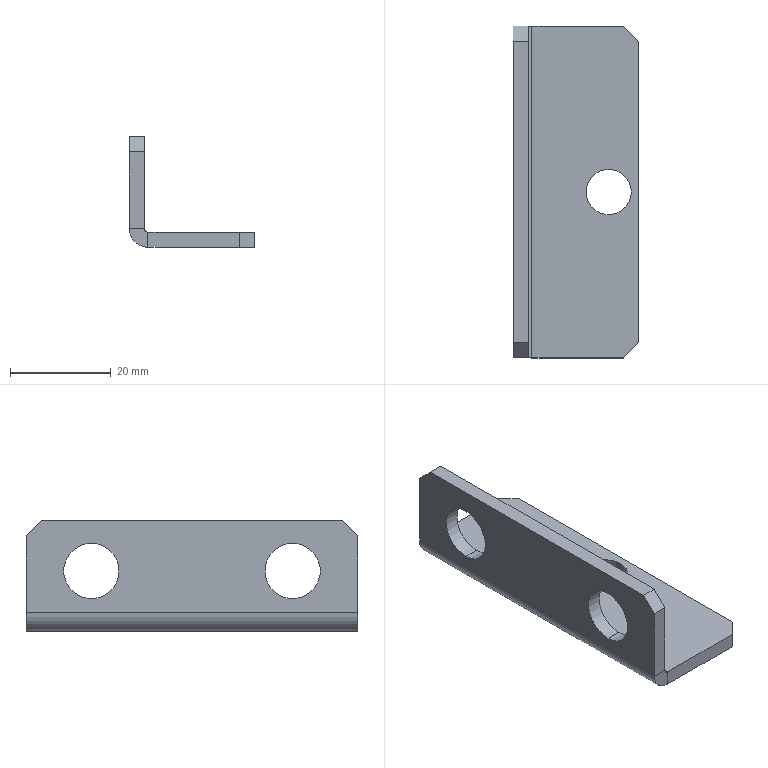Part | SolidWorks | features HoleWzd 2, 3DProfileFeature 1, BreakCorner 1, EdgeFlange 1, FlatPattern 1, SMBaseFlange 1, SheetMetal 1 | 1 solid | 24 faces | box 25 x 66 x 22 mm | volume 7707 mm3 | plane 16 | cylinder 8 | commonest cylinder face diameters 11 x4 9 x2 1.473 x1 7.473 x1
STEP:
#1=CARTESIAN_POINT('',(11.,0.,-3.));
#2=VERTEX_POINT('',#1);
#3=CARTESIAN_POINT('',(2.,0.,-3.));
#4=VERTEX_POINT('',#3);
#5=CARTESIAN_POINT('',(6.5,0.,-3.));
#6=DIRECTION('',(0.,0.,-1.));
#7=DIRECTION('',(-1.,0.,0.));
#8=AXIS2_PLACEMENT_3D('',#5,#6,#7);
#9=CIRCLE('',#8,4.5);
#10=EDGE_CURVE('',#2,#4,#9,.T.);
#11=ORIENTED_EDGE('',*,*,#10,.T.);
#12=CARTESIAN_POINT('',(2.,0.,0.));
#13=VERTEX_POINT('',#12);
#14=CARTESIAN_POINT('',(2.,0.,0.));
#15=DIRECTION('',(0.,0.,1.));
#16=VECTOR('',#15,1000.);
#17=LINE('',#14,#16);
#18=EDGE_CURVE('',#4,#13,#17,.T.);
#19=ORIENTED_EDGE('',*,*,#18,.T.);
#20=CARTESIAN_POINT('',(11.,0.,0.));
#21=VERTEX_POINT('',#20);
#22=CARTESIAN_POINT('',(6.5,0.,0.));
#23=DIRECTION('',(0.,0.,1.));
#24=DIRECTION('',(1.,0.,0.));
#25=AXIS2_PLACEMENT_3D('',#22,#23,#24);
#26=CIRCLE('',#25,4.5);
#27=EDGE_CURVE('',#13,#21,#26,.T.);
#28=ORIENTED_EDGE('',*,*,#27,.T.);
#29=CARTESIAN_POINT('',(11.,0.,0.));
#30=DIRECTION('',(0.,0.,1.));
#31=VECTOR('',#30,1000.);
#32=LINE('',#29,#31);
#33=EDGE_CURVE('',#2,#21,#32,.T.);
#34=ORIENTED_EDGE('',*,*,#33,.F.);
#35=EDGE_LOOP('',(#11,#19,#28,#34));
#36=FACE_OUTER_BOUND('',#35,.T.);
#37=CARTESIAN_POINT('',(6.5,0.,0.));
#38=DIRECTION('',(0.,0.,1.));
#39=DIRECTION('',(1.,0.,0.));
#40=AXIS2_PLACEMENT_3D('',#37,#38,#39);
#41=CYLINDRICAL_SURFACE('',#40,4.5);
#42=ADVANCED_FACE('',(#36),#41,.F.);
#43=CARTESIAN_POINT('',(-12.5,20.,14.5));
#44=VERTEX_POINT('',#43);
#45=CARTESIAN_POINT('',(-12.5,20.,3.5));
#46=VERTEX_POINT('',#45);
#47=CARTESIAN_POINT('',(-12.5,20.,9.));
#48=DIRECTION('',(1.,0.,0.));
#49=DIRECTION('',(0.,0.,-1.));
#50=AXIS2_PLACEMENT_3D('',#47,#48,#49);
#51=CIRCLE('',#50,5.5);
#52=EDGE_CURVE('',#44,#46,#51,.T.);
#53=ORIENTED_EDGE('',*,*,#52,.F.);
#54=CARTESIAN_POINT('',(-9.5,20.,14.5));
#55=VERTEX_POINT('',#54);
#56=CARTESIAN_POINT('',(-9.5,20.,14.5));
#57=DIRECTION('',(1.,0.,0.));
#58=VECTOR('',#57,1000.);
#59=LINE('',#56,#58);
#60=EDGE_CURVE('',#44,#55,#59,.T.);
#61=ORIENTED_EDGE('',*,*,#60,.T.);
#62=CARTESIAN_POINT('',(-9.5,20.,3.5));
#63=VERTEX_POINT('',#62);
#64=CARTESIAN_POINT('',(-9.5,20.,9.));
#65=DIRECTION('',(1.,0.,0.));
#66=DIRECTION('',(0.,0.,-1.));
#67=AXIS2_PLACEMENT_3D('',#64,#65,#66);
#68=CIRCLE('',#67,5.5);
#69=EDGE_CURVE('',#55,#63,#68,.T.);
#70=ORIENTED_EDGE('',*,*,#69,.T.);
#71=CARTESIAN_POINT('',(-9.5,20.,3.5));
#72=DIRECTION('',(1.,0.,0.));
#73=VECTOR('',#72,1000.);
#74=LINE('',#71,#73);
#75=EDGE_CURVE('',#46,#63,#74,.T.);
#76=ORIENTED_EDGE('',*,*,#75,.F.);
#77=EDGE_LOOP('',(#53,#61,#70,#76));
#78=FACE_OUTER_BOUND('',#77,.T.);
#79=CARTESIAN_POINT('',(-9.5,20.,9.));
#80=DIRECTION('',(1.,0.,0.));
#81=DIRECTION('',(0.,0.,-1.));
#82=AXIS2_PLACEMENT_3D('',#79,#80,#81);
#83=CYLINDRICAL_SURFACE('',#82,5.5);
#84=ADVANCED_FACE('',(#78),#83,.F.);
#85=CARTESIAN_POINT('',(-12.5,-20.,14.5));
#86=VERTEX_POINT('',#85);
#87=CARTESIAN_POINT('',(-12.5,-20.,3.5));
#88=VERTEX_POINT('',#87);
#89=CARTESIAN_POINT('',(-12.5,-20.,9.));
#90=DIRECTION('',(1.,0.,0.));
#91=DIRECTION('',(0.,0.,-1.));
#92=AXIS2_PLACEMENT_3D('',#89,#90,#91);
#93=CIRCLE('',#92,5.5);
#94=EDGE_CURVE('',#86,#88,#93,.T.);
#95=ORIENTED_EDGE('',*,*,#94,.F.);
#96=CARTESIAN_POINT('',(-9.5,-20.,14.5));
#97=VERTEX_POINT('',#96);
#98=CARTESIAN_POINT('',(-9.5,-20.,14.5));
#99=DIRECTION('',(1.,0.,0.));
#100=VECTOR('',#99,1000.);
#101=LINE('',#98,#100);
#102=EDGE_CURVE('',#86,#97,#101,.T.);
#103=ORIENTED_EDGE('',*,*,#102,.T.);
#104=CARTESIAN_POINT('',(-9.5,-20.,3.5));
#105=VERTEX_POINT('',#104);
#106=CARTESIAN_POINT('',(-9.5,-20.,9.));
#107=DIRECTION('',(1.,0.,0.));
#108=DIRECTION('',(0.,0.,-1.));
#109=AXIS2_PLACEMENT_3D('',#106,#107,#108);
#110=CIRCLE('',#109,5.5);
#111=EDGE_CURVE('',#97,#105,#110,.T.);
#112=ORIENTED_EDGE('',*,*,#111,.T.);
#113=CARTESIAN_POINT('',(-9.5,-20.,3.5));
#114=DIRECTION('',(1.,0.,0.));
#115=VECTOR('',#114,1000.);
#116=LINE('',#113,#115);
#117=EDGE_CURVE('',#88,#105,#116,.T.);
#118=ORIENTED_EDGE('',*,*,#117,.F.);
#119=EDGE_LOOP('',(#95,#103,#112,#118));
#120=FACE_OUTER_BOUND('',#119,.T.);
#121=CARTESIAN_POINT('',(-9.5,-20.,9.));
#122=DIRECTION('',(1.,0.,0.));
#123=DIRECTION('',(0.,0.,-1.));
#124=AXIS2_PLACEMENT_3D('',#121,#122,#123);
#125=CYLINDRICAL_SURFACE('',#124,5.5);
#126=ADVANCED_FACE('',(#120),#125,.F.);
#127=CARTESIAN_POINT('',(-8.763,-33.,-3.));
#128=VERTEX_POINT('',#127);
#129=CARTESIAN_POINT('',(9.5,-33.,-3.));
#130=VERTEX_POINT('',#129);
#131=CARTESIAN_POINT('',(-12.5,-33.,-3.));
#132=DIRECTION('',(1.,0.,0.));
#133=VECTOR('',#132,1000.);
#134=LINE('',#131,#133);
#135=EDGE_CURVE('',#128,#130,#134,.T.);
#136=ORIENTED_EDGE('',*,*,#135,.T.);
#137=CARTESIAN_POINT('',(9.5,-33.,0.));
#138=VERTEX_POINT('',#137);
#139=CARTESIAN_POINT('',(9.5,-33.,-3.));
#140=DIRECTION('',(0.,0.,1.));
#141=VECTOR('',#140,1000.);
#142=LINE('',#139,#141);
#143=EDGE_CURVE('',#130,#138,#142,.T.);
#144=ORIENTED_EDGE('',*,*,#143,.T.);
#145=CARTESIAN_POINT('',(-8.763,-33.,0.));
#146=VERTEX_POINT('',#145);
#147=CARTESIAN_POINT('',(-12.5,-33.,0.));
#148=DIRECTION('',(1.,0.,0.));
#149=VECTOR('',#148,1000.);
#150=LINE('',#147,#149);
#151=EDGE_CURVE('',#146,#138,#150,.T.);
#152=ORIENTED_EDGE('',*,*,#151,.F.);
#153=CARTESIAN_POINT('',(-8.763,-33.,0.));
#154=DIRECTION('',(0.,0.,-1.));
#155=VECTOR('',#154,1000.);
#156=LINE('',#153,#155);
#157=EDGE_CURVE('',#146,#128,#156,.T.);
#158=ORIENTED_EDGE('',*,*,#157,.T.);
#159=EDGE_LOOP('',(#136,#144,#152,#158));
#160=FACE_OUTER_BOUND('',#159,.T.);
#161=CARTESIAN_POINT('',(-12.5,-33.,-3.));
#162=DIRECTION('',(0.,-1.,0.));
#163=DIRECTION('',(0.,0.,-1.));
#164=AXIS2_PLACEMENT_3D('',#161,#162,#163);
#165=PLANE('',#164);
#166=ADVANCED_FACE('',(#160),#165,.T.);
#167=ORIENTED_EDGE('',*,*,#10,.F.);
#168=CARTESIAN_POINT('',(6.5,0.,-3.));
#169=DIRECTION('',(0.,0.,-1.));
#170=DIRECTION('',(-1.,0.,0.));
#171=AXIS2_PLACEMENT_3D('',#168,#169,#170);
#172=CIRCLE('',#171,4.5);
#173=EDGE_CURVE('',#4,#2,#172,.T.);
#174=ORIENTED_EDGE('',*,*,#173,.F.);
#175=EDGE_LOOP('',(#167,#174));
#176=FACE_BOUND('',#175,.T.);
#177=CARTESIAN_POINT('',(9.5,33.,-3.));
#178=VERTEX_POINT('',#177);
#179=CARTESIAN_POINT('',(-8.763,33.,-3.));
#180=VERTEX_POINT('',#179);
#181=CARTESIAN_POINT('',(-12.5,33.,-3.));
#182=DIRECTION('',(-1.,0.,0.));
#183=VECTOR('',#182,1000.);
#184=LINE('',#181,#183);
#185=EDGE_CURVE('',#178,#180,#184,.T.);
#186=ORIENTED_EDGE('',*,*,#185,.F.);
#187=CARTESIAN_POINT('',(12.5,30.,-3.));
#188=VERTEX_POINT('',#187);
#189=CARTESIAN_POINT('',(21.25,21.25,-3.));
#190=DIRECTION('',(0.7071,-0.7071,0.));
#191=VECTOR('',#190,1000.);
#192=LINE('',#189,#191);
#193=EDGE_CURVE('',#178,#188,#192,.T.);
#194=ORIENTED_EDGE('',*,*,#193,.T.);
#195=CARTESIAN_POINT('',(12.5,-30.,-3.));
#196=VERTEX_POINT('',#195);
#197=CARTESIAN_POINT('',(12.5,-33.,-3.));
#198=DIRECTION('',(0.,1.,0.));
#199=VECTOR('',#198,1000.);
#200=LINE('',#197,#199);
#201=EDGE_CURVE('',#196,#188,#200,.T.);
#202=ORIENTED_EDGE('',*,*,#201,.F.);
#203=CARTESIAN_POINT('',(21.25,-21.25,-3.));
#204=DIRECTION('',(-0.7071,-0.7071,0.));
#205=VECTOR('',#204,1000.);
#206=LINE('',#203,#205);
#207=EDGE_CURVE('',#196,#130,#206,.T.);
#208=ORIENTED_EDGE('',*,*,#207,.T.);
#209=ORIENTED_EDGE('',*,*,#135,.F.);
#210=CARTESIAN_POINT('',(-8.763,-33.,-3.));
#211=DIRECTION('',(0.,1.,0.));
#212=VECTOR('',#211,1000.);
#213=LINE('',#210,#212);
#214=EDGE_CURVE('',#128,#180,#213,.T.);
#215=ORIENTED_EDGE('',*,*,#214,.T.);
#216=EDGE_LOOP('',(#186,#194,#202,#208,#209,#215));
#217=FACE_OUTER_BOUND('',#216,.T.);
#218=CARTESIAN_POINT('',(0.,0.,-3.));
#219=DIRECTION('',(0.,0.,-1.));
#220=DIRECTION('',(-1.,0.,0.));
#221=AXIS2_PLACEMENT_3D('',#218,#219,#220);
#222=PLANE('',#221);
#223=ADVANCED_FACE('',(#176,#217),#222,.T.);
#224=CARTESIAN_POINT('',(6.5,0.,0.));
#225=DIRECTION('',(0.,0.,1.));
#226=DIRECTION('',(1.,0.,0.));
#227=AXIS2_PLACEMENT_3D('',#224,#225,#226);
#228=CIRCLE('',#227,4.5);
#229=EDGE_CURVE('',#21,#13,#228,.T.);
#230=ORIENTED_EDGE('',*,*,#229,.F.);
#231=ORIENTED_EDGE('',*,*,#27,.F.);
#232=EDGE_LOOP('',(#230,#231));
#233=FACE_BOUND('',#232,.T.);
#234=CARTESIAN_POINT('',(12.5,-30.,0.));
#235=VERTEX_POINT('',#234);
#236=CARTESIAN_POINT('',(12.5,30.,0.));
#237=VERTEX_POINT('',#236);
#238=CARTESIAN_POINT('',(12.5,-33.,0.));
#239=DIRECTION('',(0.,1.,0.));
#240=VECTOR('',#239,1000.);
#241=LINE('',#238,#240);
#242=EDGE_CURVE('',#235,#237,#241,.T.);
#243=ORIENTED_EDGE('',*,*,#242,.T.);
#244=CARTESIAN_POINT('',(9.5,33.,0.));
#245=VERTEX_POINT('',#244);
#246=CARTESIAN_POINT('',(12.5,30.,0.));
#247=DIRECTION('',(-0.7071,0.7071,0.));
#248=VECTOR('',#247,1000.);
#249=LINE('',#246,#248);
#250=EDGE_CURVE('',#237,#245,#249,.T.);
#251=ORIENTED_EDGE('',*,*,#250,.T.);
#252=CARTESIAN_POINT('',(-8.763,33.,0.));
#253=VERTEX_POINT('',#252);
#254=CARTESIAN_POINT('',(-12.5,33.,0.));
#255=DIRECTION('',(-1.,0.,0.));
#256=VECTOR('',#255,1000.);
#257=LINE('',#254,#256);
#258=EDGE_CURVE('',#245,#253,#257,.T.);
#259=ORIENTED_EDGE('',*,*,#258,.T.);
#260=CARTESIAN_POINT('',(-8.763,-33.,0.));
#261=DIRECTION('',(0.,1.,0.));
#262=VECTOR('',#261,1000.);
#263=LINE('',#260,#262);
#264=EDGE_CURVE('',#146,#253,#263,.T.);
#265=ORIENTED_EDGE('',*,*,#264,.F.);
#266=ORIENTED_EDGE('',*,*,#151,.T.);
#267=CARTESIAN_POINT('',(9.5,-33.,0.));
#268=DIRECTION('',(0.7071,0.7071,0.));
#269=VECTOR('',#268,1000.);
#270=LINE('',#267,#269);
#271=EDGE_CURVE('',#138,#235,#270,.T.);
#272=ORIENTED_EDGE('',*,*,#271,.T.);
#273=EDGE_LOOP('',(#243,#251,#259,#265,#266,#272));
#274=FACE_OUTER_BOUND('',#273,.T.);
#275=CARTESIAN_POINT('',(0.,0.,0.));
#276=DIRECTION('',(0.,0.,-1.));
#277=DIRECTION('',(-1.,0.,0.));
#278=AXIS2_PLACEMENT_3D('',#275,#276,#277);
#279=PLANE('',#278);
#280=ADVANCED_FACE('',(#233,#274),#279,.F.);
#281=ORIENTED_EDGE('',*,*,#201,.T.);
#282=CARTESIAN_POINT('',(12.5,30.,-3.));
#283=DIRECTION('',(0.,0.,1.));
#284=VECTOR('',#283,1000.);
#285=LINE('',#282,#284);
#286=EDGE_CURVE('',#188,#237,#285,.T.);
#287=ORIENTED_EDGE('',*,*,#286,.T.);
#288=ORIENTED_EDGE('',*,*,#242,.F.);
#289=CARTESIAN_POINT('',(12.5,-30.,-3.));
#290=DIRECTION('',(0.,0.,-1.));
#291=VECTOR('',#290,1000.);
#292=LINE('',#289,#291);
#293=EDGE_CURVE('',#235,#196,#292,.T.);
#294=ORIENTED_EDGE('',*,*,#293,.T.);
#295=EDGE_LOOP('',(#281,#287,#288,#294));
#296=FACE_OUTER_BOUND('',#295,.T.);
#297=CARTESIAN_POINT('',(12.5,-33.,-3.));
#298=DIRECTION('',(1.,0.,0.));
#299=DIRECTION('',(0.,0.,-1.));
#300=AXIS2_PLACEMENT_3D('',#297,#298,#299);
#301=PLANE('',#300);
#302=ADVANCED_FACE('',(#296),#301,.T.);
#303=ORIENTED_EDGE('',*,*,#258,.F.);
#304=CARTESIAN_POINT('',(9.5,33.,-3.));
#305=DIRECTION('',(0.,0.,-1.));
#306=VECTOR('',#305,1000.);
#307=LINE('',#304,#306);
#308=EDGE_CURVE('',#245,#178,#307,.T.);
#309=ORIENTED_EDGE('',*,*,#308,.T.);
#310=ORIENTED_EDGE('',*,*,#185,.T.);
#311=CARTESIAN_POINT('',(-8.763,33.,0.));
#312=DIRECTION('',(0.,0.,-1.));
#313=VECTOR('',#312,1000.);
#314=LINE('',#311,#313);
#315=EDGE_CURVE('',#253,#180,#314,.T.);
#316=ORIENTED_EDGE('',*,*,#315,.F.);
#317=EDGE_LOOP('',(#303,#309,#310,#316));
#318=FACE_OUTER_BOUND('',#317,.T.);
#319=CARTESIAN_POINT('',(-12.5,33.,-3.));
#320=DIRECTION('',(0.,1.,0.));
#321=DIRECTION('',(0.,0.,1.));
#322=AXIS2_PLACEMENT_3D('',#319,#320,#321);
#323=PLANE('',#322);
#324=ADVANCED_FACE('',(#318),#323,.T.);
#325=CARTESIAN_POINT('',(-9.5,33.,0.7366));
#326=VERTEX_POINT('',#325);
#327=CARTESIAN_POINT('',(-12.5,33.,0.7366));
#328=VERTEX_POINT('',#327);
#329=CARTESIAN_POINT('',(-12.5,33.,0.7366));
#330=DIRECTION('',(-1.,0.,0.));
#331=VECTOR('',#330,1000.);
#332=LINE('',#329,#331);
#333=EDGE_CURVE('',#326,#328,#332,.T.);
#334=ORIENTED_EDGE('',*,*,#333,.F.);
#335=CARTESIAN_POINT('',(-8.763,33.,0.7366));
#336=DIRECTION('',(0.,1.,0.));
#337=DIRECTION('',(0.,0.,-1.));
#338=AXIS2_PLACEMENT_3D('',#335,#336,#337);
#339=CIRCLE('',#338,0.7366);
#340=EDGE_CURVE('',#253,#326,#339,.T.);
#341=ORIENTED_EDGE('',*,*,#340,.F.);
#342=ORIENTED_EDGE('',*,*,#315,.T.);
#343=CARTESIAN_POINT('',(-8.763,33.,0.7366));
#344=DIRECTION('',(0.,1.,0.));
#345=DIRECTION('',(0.,0.,-1.));
#346=AXIS2_PLACEMENT_3D('',#343,#344,#345);
#347=CIRCLE('',#346,3.737);
#348=EDGE_CURVE('',#180,#328,#347,.T.);
#349=ORIENTED_EDGE('',*,*,#348,.T.);
#350=EDGE_LOOP('',(#334,#341,#342,#349));
#351=FACE_OUTER_BOUND('',#350,.T.);
#352=CARTESIAN_POINT('',(-8.763,33.,0.7366));
#353=DIRECTION('',(0.,1.,0.));
#354=DIRECTION('',(0.,0.,1.));
#355=AXIS2_PLACEMENT_3D('',#352,#353,#354);
#356=PLANE('',#355);
#357=ADVANCED_FACE('',(#351),#356,.T.);
#358=CARTESIAN_POINT('',(-9.5,-33.,0.7366));
#359=VERTEX_POINT('',#358);
#360=CARTESIAN_POINT('',(-8.763,-33.,0.7366));
#361=DIRECTION('',(0.,-1.,0.));
#362=DIRECTION('',(0.,0.,-1.));
#363=AXIS2_PLACEMENT_3D('',#360,#361,#362);
#364=CIRCLE('',#363,0.7366);
#365=EDGE_CURVE('',#359,#146,#364,.T.);
#366=ORIENTED_EDGE('',*,*,#365,.F.);
#367=CARTESIAN_POINT('',(-12.5,-33.,0.7366));
#368=VERTEX_POINT('',#367);
#369=CARTESIAN_POINT('',(-9.5,-33.,0.7366));
#370=DIRECTION('',(-1.,0.,0.));
#371=VECTOR('',#370,1000.);
#372=LINE('',#369,#371);
#373=EDGE_CURVE('',#359,#368,#372,.T.);
#374=ORIENTED_EDGE('',*,*,#373,.T.);
#375=CARTESIAN_POINT('',(-8.763,-33.,0.7366));
#376=DIRECTION('',(0.,-1.,0.));
#377=DIRECTION('',(0.,0.,-1.));
#378=AXIS2_PLACEMENT_3D('',#375,#376,#377);
#379=CIRCLE('',#378,3.737);
#380=EDGE_CURVE('',#368,#128,#379,.T.);
#381=ORIENTED_EDGE('',*,*,#380,.T.);
#382=ORIENTED_EDGE('',*,*,#157,.F.);
#383=EDGE_LOOP('',(#366,#374,#381,#382));
#384=FACE_OUTER_BOUND('',#383,.T.);
#385=CARTESIAN_POINT('',(-8.763,-33.,0.7366));
#386=DIRECTION('',(0.,1.,0.));
#387=DIRECTION('',(0.,0.,1.));
#388=AXIS2_PLACEMENT_3D('',#385,#386,#387);
#389=PLANE('',#388);
#390=ADVANCED_FACE('',(#384),#389,.F.);
#391=ORIENTED_EDGE('',*,*,#214,.F.);
#392=ORIENTED_EDGE('',*,*,#380,.F.);
#393=CARTESIAN_POINT('',(-12.5,33.,0.7366));
#394=DIRECTION('',(0.,1.,0.));
#395=VECTOR('',#394,1000.);
#396=LINE('',#393,#395);
#397=EDGE_CURVE('',#368,#328,#396,.T.);
#398=ORIENTED_EDGE('',*,*,#397,.T.);
#399=ORIENTED_EDGE('',*,*,#348,.F.);
#400=EDGE_LOOP('',(#391,#392,#398,#399));
#401=FACE_OUTER_BOUND('',#400,.T.);
#402=CARTESIAN_POINT('',(-8.763,-33.,0.7366));
#403=DIRECTION('',(0.,-1.,0.));
#404=DIRECTION('',(-1.,0.,0.));
#405=AXIS2_PLACEMENT_3D('',#402,#403,#404);
#406=CYLINDRICAL_SURFACE('',#405,3.737);
#407=ADVANCED_FACE('',(#401),#406,.T.);
#408=ORIENTED_EDGE('',*,*,#264,.T.);
#409=ORIENTED_EDGE('',*,*,#340,.T.);
#410=CARTESIAN_POINT('',(-9.5,33.,0.7366));
#411=DIRECTION('',(0.,-1.,0.));
#412=VECTOR('',#411,1000.);
#413=LINE('',#410,#412);
#414=EDGE_CURVE('',#326,#359,#413,.T.);
#415=ORIENTED_EDGE('',*,*,#414,.T.);
#416=ORIENTED_EDGE('',*,*,#365,.T.);
#417=EDGE_LOOP('',(#408,#409,#415,#416));
#418=FACE_OUTER_BOUND('',#417,.T.);
#419=CARTESIAN_POINT('',(-8.763,-33.,0.7366));
#420=DIRECTION('',(0.,-1.,0.));
#421=DIRECTION('',(-1.,0.,0.));
#422=AXIS2_PLACEMENT_3D('',#419,#420,#421);
#423=CYLINDRICAL_SURFACE('',#422,0.7366);
#424=ADVANCED_FACE('',(#418),#423,.F.);
#425=CARTESIAN_POINT('',(-9.5,-33.,16.));
#426=VERTEX_POINT('',#425);
#427=CARTESIAN_POINT('',(-9.5,-33.,19.));
#428=DIRECTION('',(0.,0.,1.));
#429=VECTOR('',#428,1000.);
#430=LINE('',#427,#429);
#431=EDGE_CURVE('',#359,#426,#430,.T.);
#432=ORIENTED_EDGE('',*,*,#431,.T.);
#433=CARTESIAN_POINT('',(-12.5,-33.,16.));
#434=VERTEX_POINT('',#433);
#435=CARTESIAN_POINT('',(-12.5,-33.,16.));
#436=DIRECTION('',(-1.,0.,0.));
#437=VECTOR('',#436,1000.);
#438=LINE('',#435,#437);
#439=EDGE_CURVE('',#426,#434,#438,.T.);
#440=ORIENTED_EDGE('',*,*,#439,.T.);
#441=CARTESIAN_POINT('',(-12.5,-33.,0.));
#442=DIRECTION('',(0.,0.,1.));
#443=VECTOR('',#442,1000.);
#444=LINE('',#441,#443);
#445=EDGE_CURVE('',#368,#434,#444,.T.);
#446=ORIENTED_EDGE('',*,*,#445,.F.);
#447=ORIENTED_EDGE('',*,*,#373,.F.);
#448=EDGE_LOOP('',(#432,#440,#446,#447));
#449=FACE_OUTER_BOUND('',#448,.T.);
#450=CARTESIAN_POINT('',(-12.5,-33.,19.));
#451=DIRECTION('',(0.,1.,0.));
#452=DIRECTION('',(0.,0.,1.));
#453=AXIS2_PLACEMENT_3D('',#450,#451,#452);
#454=PLANE('',#453);
#455=ADVANCED_FACE('',(#449),#454,.F.);
#456=CARTESIAN_POINT('',(-12.5,33.,16.));
#457=VERTEX_POINT('',#456);
#458=CARTESIAN_POINT('',(-12.5,33.,0.));
#459=DIRECTION('',(0.,0.,-1.));
#460=VECTOR('',#459,1000.);
#461=LINE('',#458,#460);
#462=EDGE_CURVE('',#457,#328,#461,.T.);
#463=ORIENTED_EDGE('',*,*,#462,.F.);
#464=CARTESIAN_POINT('',(-9.5,33.,16.));
#465=VERTEX_POINT('',#464);
#466=CARTESIAN_POINT('',(-12.5,33.,16.));
#467=DIRECTION('',(1.,0.,0.));
#468=VECTOR('',#467,1000.);
#469=LINE('',#466,#468);
#470=EDGE_CURVE('',#457,#465,#469,.T.);
#471=ORIENTED_EDGE('',*,*,#470,.T.);
#472=CARTESIAN_POINT('',(-9.5,33.,0.));
#473=DIRECTION('',(0.,0.,-1.));
#474=VECTOR('',#473,1000.);
#475=LINE('',#472,#474);
#476=EDGE_CURVE('',#465,#326,#475,.T.);
#477=ORIENTED_EDGE('',*,*,#476,.T.);
#478=ORIENTED_EDGE('',*,*,#333,.T.);
#479=EDGE_LOOP('',(#463,#471,#477,#478));
#480=FACE_OUTER_BOUND('',#479,.T.);
#481=CARTESIAN_POINT('',(-12.5,33.,0.));
#482=DIRECTION('',(0.,-1.,0.));
#483=DIRECTION('',(0.,0.,-1.));
#484=AXIS2_PLACEMENT_3D('',#481,#482,#483);
#485=PLANE('',#484);
#486=ADVANCED_FACE('',(#480),#485,.F.);
#487=CARTESIAN_POINT('',(-12.5,20.,9.));
#488=DIRECTION('',(1.,0.,0.));
#489=DIRECTION('',(0.,0.,-1.));
#490=AXIS2_PLACEMENT_3D('',#487,#488,#489);
#491=CIRCLE('',#490,5.5);
#492=EDGE_CURVE('',#46,#44,#491,.T.);
#493=ORIENTED_EDGE('',*,*,#492,.T.);
#494=ORIENTED_EDGE('',*,*,#52,.T.);
#495=EDGE_LOOP('',(#493,#494));
#496=FACE_BOUND('',#495,.T.);
#497=CARTESIAN_POINT('',(-12.5,-20.,9.));
#498=DIRECTION('',(1.,0.,0.));
#499=DIRECTION('',(0.,0.,-1.));
#500=AXIS2_PLACEMENT_3D('',#497,#498,#499);
#501=CIRCLE('',#500,5.5);
#502=EDGE_CURVE('',#88,#86,#501,.T.);
#503=ORIENTED_EDGE('',*,*,#502,.T.);
#504=ORIENTED_EDGE('',*,*,#94,.T.);
#505=EDGE_LOOP('',(#503,#504));
#506=FACE_BOUND('',#505,.T.);
#507=CARTESIAN_POINT('',(-12.5,-30.,19.));
#508=VERTEX_POINT('',#507);
#509=CARTESIAN_POINT('',(-12.5,30.,19.));
#510=VERTEX_POINT('',#509);
#511=CARTESIAN_POINT('',(-12.5,0.,19.));
#512=DIRECTION('',(0.,1.,0.));
#513=VECTOR('',#512,1000.);
#514=LINE('',#511,#513);
#515=EDGE_CURVE('',#508,#510,#514,.T.);
#516=ORIENTED_EDGE('',*,*,#515,.T.);
#517=CARTESIAN_POINT('',(-12.5,33.,16.));
#518=DIRECTION('',(0.,0.7071,-0.7071));
#519=VECTOR('',#518,1000.);
#520=LINE('',#517,#519);
#521=EDGE_CURVE('',#510,#457,#520,.T.);
#522=ORIENTED_EDGE('',*,*,#521,.T.);
#523=ORIENTED_EDGE('',*,*,#462,.T.);
#524=ORIENTED_EDGE('',*,*,#397,.F.);
#525=ORIENTED_EDGE('',*,*,#445,.T.);
#526=CARTESIAN_POINT('',(-12.5,-30.,19.));
#527=DIRECTION('',(0.,0.7071,0.7071));
#528=VECTOR('',#527,1000.);
#529=LINE('',#526,#528);
#530=EDGE_CURVE('',#434,#508,#529,.T.);
#531=ORIENTED_EDGE('',*,*,#530,.T.);
#532=EDGE_LOOP('',(#516,#522,#523,#524,#525,#531));
#533=FACE_OUTER_BOUND('',#532,.T.);
#534=CARTESIAN_POINT('',(-12.5,0.,0.));
#535=DIRECTION('',(1.,0.,0.));
#536=DIRECTION('',(0.,0.,-1.));
#537=AXIS2_PLACEMENT_3D('',#534,#535,#536);
#538=PLANE('',#537);
#539=ADVANCED_FACE('',(#496,#506,#533),#538,.F.);
#540=CARTESIAN_POINT('',(-9.5,20.,9.));
#541=DIRECTION('',(1.,0.,0.));
#542=DIRECTION('',(0.,0.,-1.));
#543=AXIS2_PLACEMENT_3D('',#540,#541,#542);
#544=CIRCLE('',#543,5.5);
#545=EDGE_CURVE('',#63,#55,#544,.T.);
#546=ORIENTED_EDGE('',*,*,#545,.F.);
#547=ORIENTED_EDGE('',*,*,#69,.F.);
#548=EDGE_LOOP('',(#546,#547));
#549=FACE_BOUND('',#548,.T.);
#550=CARTESIAN_POINT('',(-9.5,-20.,9.));
#551=DIRECTION('',(1.,0.,0.));
#552=DIRECTION('',(0.,0.,-1.));
#553=AXIS2_PLACEMENT_3D('',#550,#551,#552);
#554=CIRCLE('',#553,5.5);
#555=EDGE_CURVE('',#105,#97,#554,.T.);
#556=ORIENTED_EDGE('',*,*,#555,.F.);
#557=ORIENTED_EDGE('',*,*,#111,.F.);
#558=EDGE_LOOP('',(#556,#557));
#559=FACE_BOUND('',#558,.T.);
#560=ORIENTED_EDGE('',*,*,#476,.F.);
#561=CARTESIAN_POINT('',(-9.5,30.,19.));
#562=VERTEX_POINT('',#561);
#563=CARTESIAN_POINT('',(-9.5,24.5,24.5));
#564=DIRECTION('',(0.,-0.7071,0.7071));
#565=VECTOR('',#564,1000.);
#566=LINE('',#563,#565);
#567=EDGE_CURVE('',#465,#562,#566,.T.);
#568=ORIENTED_EDGE('',*,*,#567,.T.);
#569=CARTESIAN_POINT('',(-9.5,-30.,19.));
#570=VERTEX_POINT('',#569);
#571=CARTESIAN_POINT('',(-9.5,33.,19.));
#572=DIRECTION('',(0.,1.,0.));
#573=VECTOR('',#572,1000.);
#574=LINE('',#571,#573);
#575=EDGE_CURVE('',#570,#562,#574,.T.);
#576=ORIENTED_EDGE('',*,*,#575,.F.);
#577=CARTESIAN_POINT('',(-9.5,-24.5,24.5));
#578=DIRECTION('',(0.,-0.7071,-0.7071));
#579=VECTOR('',#578,1000.);
#580=LINE('',#577,#579);
#581=EDGE_CURVE('',#570,#426,#580,.T.);
#582=ORIENTED_EDGE('',*,*,#581,.T.);
#583=ORIENTED_EDGE('',*,*,#431,.F.);
#584=ORIENTED_EDGE('',*,*,#414,.F.);
#585=EDGE_LOOP('',(#560,#568,#576,#582,#583,#584));
#586=FACE_OUTER_BOUND('',#585,.T.);
#587=CARTESIAN_POINT('',(-9.5,0.,0.));
#588=DIRECTION('',(1.,0.,0.));
#589=DIRECTION('',(0.,0.,-1.));
#590=AXIS2_PLACEMENT_3D('',#587,#588,#589);
#591=PLANE('',#590);
#592=ADVANCED_FACE('',(#549,#559,#586),#591,.T.);
#593=ORIENTED_EDGE('',*,*,#575,.T.);
#594=CARTESIAN_POINT('',(-12.5,30.,19.));
#595=DIRECTION('',(-1.,0.,0.));
#596=VECTOR('',#595,1000.);
#597=LINE('',#594,#596);
#598=EDGE_CURVE('',#562,#510,#597,.T.);
#599=ORIENTED_EDGE('',*,*,#598,.T.);
#600=ORIENTED_EDGE('',*,*,#515,.F.);
#601=CARTESIAN_POINT('',(-12.5,-30.,19.));
#602=DIRECTION('',(1.,0.,0.));
#603=VECTOR('',#602,1000.);
#604=LINE('',#601,#603);
#605=EDGE_CURVE('',#508,#570,#604,.T.);
#606=ORIENTED_EDGE('',*,*,#605,.T.);
#607=EDGE_LOOP('',(#593,#599,#600,#606));
#608=FACE_OUTER_BOUND('',#607,.T.);
#609=CARTESIAN_POINT('',(-12.5,33.,19.));
#610=DIRECTION('',(0.,0.,-1.));
#611=DIRECTION('',(-1.,0.,0.));
#612=AXIS2_PLACEMENT_3D('',#609,#610,#611);
#613=PLANE('',#612);
#614=ADVANCED_FACE('',(#608),#613,.F.);
#615=ORIENTED_EDGE('',*,*,#530,.F.);
#616=ORIENTED_EDGE('',*,*,#439,.F.);
#617=ORIENTED_EDGE('',*,*,#581,.F.);
#618=ORIENTED_EDGE('',*,*,#605,.F.);
#619=EDGE_LOOP('',(#615,#616,#617,#618));
#620=FACE_OUTER_BOUND('',#619,.T.);
#621=CARTESIAN_POINT('',(-12.5,-30.,19.));
#622=DIRECTION('',(0.,0.7071,-0.7071));
#623=DIRECTION('',(1.,0.,0.));
#624=AXIS2_PLACEMENT_3D('',#621,#622,#623);
#625=PLANE('',#624);
#626=ADVANCED_FACE('',(#620),#625,.F.);
#627=ORIENTED_EDGE('',*,*,#521,.F.);
#628=ORIENTED_EDGE('',*,*,#598,.F.);
#629=ORIENTED_EDGE('',*,*,#567,.F.);
#630=ORIENTED_EDGE('',*,*,#470,.F.);
#631=EDGE_LOOP('',(#627,#628,#629,#630));
#632=FACE_OUTER_BOUND('',#631,.T.);
#633=CARTESIAN_POINT('',(-12.5,33.,16.));
#634=DIRECTION('',(0.,-0.7071,-0.7071));
#635=DIRECTION('',(1.,0.,0.));
#636=AXIS2_PLACEMENT_3D('',#633,#634,#635);
#637=PLANE('',#636);
#638=ADVANCED_FACE('',(#632),#637,.F.);
#639=ORIENTED_EDGE('',*,*,#207,.F.);
#640=ORIENTED_EDGE('',*,*,#293,.F.);
#641=ORIENTED_EDGE('',*,*,#271,.F.);
#642=ORIENTED_EDGE('',*,*,#143,.F.);
#643=EDGE_LOOP('',(#639,#640,#641,#642));
#644=FACE_OUTER_BOUND('',#643,.T.);
#645=CARTESIAN_POINT('',(9.5,-33.,-3.));
#646=DIRECTION('',(-0.7071,0.7071,0.));
#647=DIRECTION('',(0.,0.,1.));
#648=AXIS2_PLACEMENT_3D('',#645,#646,#647);
#649=PLANE('',#648);
#650=ADVANCED_FACE('',(#644),#649,.F.);
#651=ORIENTED_EDGE('',*,*,#193,.F.);
#652=ORIENTED_EDGE('',*,*,#308,.F.);
#653=ORIENTED_EDGE('',*,*,#250,.F.);
#654=ORIENTED_EDGE('',*,*,#286,.F.);
#655=EDGE_LOOP('',(#651,#652,#653,#654));
#656=FACE_OUTER_BOUND('',#655,.T.);
#657=CARTESIAN_POINT('',(12.5,30.,-3.));
#658=DIRECTION('',(-0.7071,-0.7071,0.));
#659=DIRECTION('',(0.,0.,1.));
#660=AXIS2_PLACEMENT_3D('',#657,#658,#659);
#661=PLANE('',#660);
#662=ADVANCED_FACE('',(#656),#661,.F.);
#663=ORIENTED_EDGE('',*,*,#102,.F.);
#664=ORIENTED_EDGE('',*,*,#502,.F.);
#665=ORIENTED_EDGE('',*,*,#117,.T.);
#666=ORIENTED_EDGE('',*,*,#555,.T.);
#667=EDGE_LOOP('',(#663,#664,#665,#666));
#668=FACE_OUTER_BOUND('',#667,.T.);
#669=CARTESIAN_POINT('',(-9.5,-20.,9.));
#670=DIRECTION('',(1.,0.,0.));
#671=DIRECTION('',(0.,0.,-1.));
#672=AXIS2_PLACEMENT_3D('',#669,#670,#671);
#673=CYLINDRICAL_SURFACE('',#672,5.5);
#674=ADVANCED_FACE('',(#668),#673,.F.);
#675=ORIENTED_EDGE('',*,*,#60,.F.);
#676=ORIENTED_EDGE('',*,*,#492,.F.);
#677=ORIENTED_EDGE('',*,*,#75,.T.);
#678=ORIENTED_EDGE('',*,*,#545,.T.);
#679=EDGE_LOOP('',(#675,#676,#677,#678));
#680=FACE_OUTER_BOUND('',#679,.T.);
#681=CARTESIAN_POINT('',(-9.5,20.,9.));
#682=DIRECTION('',(1.,0.,0.));
#683=DIRECTION('',(0.,0.,-1.));
#684=AXIS2_PLACEMENT_3D('',#681,#682,#683);
#685=CYLINDRICAL_SURFACE('',#684,5.5);
#686=ADVANCED_FACE('',(#680),#685,.F.);
#687=ORIENTED_EDGE('',*,*,#18,.F.);
#688=ORIENTED_EDGE('',*,*,#173,.T.);
#689=ORIENTED_EDGE('',*,*,#33,.T.);
#690=ORIENTED_EDGE('',*,*,#229,.T.);
#691=EDGE_LOOP('',(#687,#688,#689,#690));
#692=FACE_OUTER_BOUND('',#691,.T.);
#693=CARTESIAN_POINT('',(6.5,0.,0.));
#694=DIRECTION('',(0.,0.,1.));
#695=DIRECTION('',(1.,0.,0.));
#696=AXIS2_PLACEMENT_3D('',#693,#694,#695);
#697=CYLINDRICAL_SURFACE('',#696,4.5);
#698=ADVANCED_FACE('',(#692),#697,.F.);
#699=CLOSED_SHELL('',(#42,#84,#126,#166,#223,#280,#302,#324,#357,#390,#407,#424,#455,#486,#539,#592,#614,#626,#638,#650,#662,#674,#686,#698));
#700=MANIFOLD_SOLID_BREP('',#699);
#701=CARTESIAN_POINT('',(0.,0.,0.));
#702=DIRECTION('',(0.,0.,1.));
#703=DIRECTION('',(1.,0.,0.));
#704=AXIS2_PLACEMENT_3D('',#701,#702,#703);
#705=(LENGTH_UNIT()NAMED_UNIT(*)SI_UNIT(.MILLI.,.METRE.));
#706=UNCERTAINTY_MEASURE_WITH_UNIT(LENGTH_MEASURE(0.00001),#705,'','');
#707=(NAMED_UNIT(*)PLANE_ANGLE_UNIT()SI_UNIT($,.RADIAN.));
#708=(NAMED_UNIT(*)SI_UNIT($,.STERADIAN.)SOLID_ANGLE_UNIT());
#709=(GEOMETRIC_REPRESENTATION_CONTEXT(3)GLOBAL_UNCERTAINTY_ASSIGNED_CONTEXT((#706))GLOBAL_UNIT_ASSIGNED_CONTEXT((#705,#707,#708))REPRESENTATION_CONTEXT('',''));
#710=ADVANCED_BREP_SHAPE_REPRESENTATION('',(#700,#704),#709);